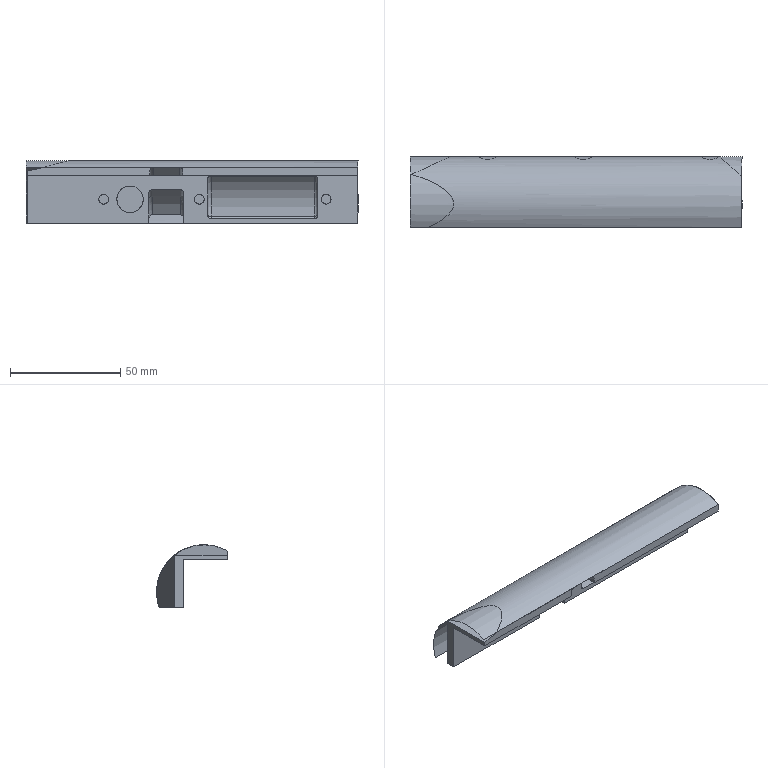NC program | Mastercam | posted with a generic post
Lines 25226 to 26102 of 52802:
(3 BM/BNOS |TOOL - 1|DIA. OFF. - 1|LEN. - 1|TOOL DIA. - 3.)
N1018 T1 M6
N1020 G0 G54 G90 X-6.118 Y-15.182 C0. B0. S6000 M3
N1022 G43 H1 Z50.
N1024 Z-20.248
N1026 G1 X-5.975 Y-15.17 Z-20.25 F2000.
N1028 X-5.578 Y-15.018 Z-20.258
N1030 X-5.28 Y-14.715 Z-20.265
N1032 X-5.135 Y-14.315 Z-20.273
N1034 X-5.126 Y-14.173 Z-20.275
N1036 X-5.128 Y-13.966
N1038 X-5.129 Y-.665
N1040 G3 X-5.128 Y-.638 I-.614 J.027
N1042 X-5.49 Y-.078 I-.615
N1044 G1 X-5.772 Y-.061
N1046 X-18.564 Y-.069
N1048 G3 X-18.907 Y-.388 I.16 J-.517
N1050 X-18.967 Y-.811 I1.449 J-.423
N1052 X-18.962 Y-.943 I1.509
N1054 G1 Y-13.966
N1056 X-18.964 Y-14.173
N1058 X-18.955 Y-14.315 Z-20.273
N1060 X-18.81 Y-14.715 Z-20.265
N1062 X-18.512 Y-15.018 Z-20.258
N1064 X-18.115 Y-15.17 Z-20.25
N1066 X-17.972 Y-15.182 Z-20.248
N1068 G0 Z50.
N1070 X-6.391 Y-15.18
N1072 Z-20.546
N1074 G1 X-6.249 Y-15.169 Z-20.548
N1076 X-5.852 Y-15.017 Z-20.556
N1078 X-5.553 Y-14.715 Z-20.563
N1080 X-5.407 Y-14.315 Z-20.571
N1082 X-5.398 Y-14.173 Z-20.573
N1084 X-5.399 Y-13.966
N1086 X-5.423 Y-.523
N1088 G3 X-5.628 Y-.332 I-.236 J-.049
N1090 G1 X-18.441
N1092 G3 X-18.667 Y-.518 I.012 J-.244
N1094 G1 X-18.689 Y-.665
N1096 X-18.692 Y-14.173
N1098 X-18.682 Y-14.315 Z-20.571
N1100 X-18.534 Y-14.714 Z-20.563
N1102 X-18.233 Y-15.014 Z-20.556
N1104 X-17.835 Y-15.163 Z-20.548
N1106 X-17.693 Y-15.173 Z-20.546
N1108 G0 Z50.
N1110 X-6.557 Y-15.179
N1112 Z-20.844
N1114 G1 X-6.415 Y-15.168 Z-20.847
N1116 X-6.017 Y-15.017 Z-20.854
N1118 X-5.719 Y-14.715 Z-20.862
N1120 X-5.573 Y-14.315 Z-20.869
N1122 X-5.563 Y-14.173 Z-20.872
N1124 X-5.564 Y-13.966
N1126 X-5.57 Y-.618
N1128 X-5.62 Y-.499
N1130 X-18.467 Y-.498
N1132 G3 X-18.524 Y-.651 I.176 J-.153
N1134 G1 Y-.665
N1136 X-18.526 Y-7.977
N1138 X-18.527 Y-14.173
N1140 X-18.517 Y-14.315 Z-20.869
N1142 X-18.369 Y-14.714 Z-20.862
N1144 X-18.068 Y-15.014 Z-20.854
N1146 X-17.67 Y-15.163 Z-20.847
N1148 X-17.527 Y-15.173 Z-20.844
N1150 G0 Z50.
N1152 X-6.65 Y-15.179
N1154 Z-21.142
N1156 G1 X-6.508 Y-15.168 Z-21.145
N1158 X-6.11 Y-15.017 Z-21.152
N1160 X-5.812 Y-14.714 Z-21.16
N1162 X-5.665 Y-14.315 Z-21.167
N1164 X-5.656 Y-14.173 Z-21.17
N1166 X-5.657 Y-13.966
N1168 X-5.662 Y-.633
N1170 X-18.428
N1172 X-18.441 Y-14.173
N1174 X-18.431 Y-14.315 Z-21.167
N1176 X-18.283 Y-14.714 Z-21.16
N1178 X-17.982 Y-15.015 Z-21.152
N1180 X-17.584 Y-15.164 Z-21.145
N1182 X-17.442 Y-15.174 Z-21.142
N1184 G0 Z50.
N1186 X-6.683 Y-15.179
N1188 Z-21.44
N1190 G1 X-6.541 Y-15.168 Z-21.443
N1192 X-6.143 Y-15.017 Z-21.45
N1194 X-5.844 Y-14.714 Z-21.458
N1196 X-5.698 Y-14.315 Z-21.465
N1198 X-5.689 Y-14.173 Z-21.468
N1200 X-5.69 Y-13.966
N1202 Y-.768
N1204 X-18.398
N1206 X-18.402 Y-14.173
N1208 X-18.392 Y-14.315 Z-21.465
N1210 X-18.243 Y-14.714 Z-21.458
N1212 X-17.943 Y-15.014 Z-21.45
N1214 X-17.544 Y-15.163 Z-21.443
N1216 X-17.402 Y-15.173 Z-21.44
N1218 G0 Z50.
N1220 X-6.688
N1222 Z-21.739
N1224 G1 X-6.546 Y-15.163 Z-21.741
N1226 X-6.148 Y-15.014 Z-21.749
N1228 X-5.847 Y-14.714 Z-21.756
N1230 X-5.699 Y-14.315 Z-21.764
N1232 X-5.688 Y-14.173 Z-21.766
N1234 X-5.69 Y-8.182
N1236 X-5.691 Y-.909
N1238 X-18.4 Y-.915
N1240 X-18.401 Y-14.173
N1242 X-18.392 Y-14.315 Z-21.764
N1244 X-18.245 Y-14.714 Z-21.756
N1246 X-17.947 Y-15.017 Z-21.749
N1248 X-17.549 Y-15.168 Z-21.741
N1250 X-17.407 Y-15.179 Z-21.739
N1252 G0 Z50.
N1254 X-6.688 Y-15.173
N1256 Z-22.037
N1258 G1 X-6.546 Y-15.163 Z-22.039
N1260 X-6.148 Y-15.014 Z-22.047
N1262 X-5.847 Y-14.714 Z-22.054
N1264 X-5.699 Y-14.315 Z-22.062
N1266 X-5.688 Y-14.173 Z-22.064
N1268 X-5.691 Y-1.059
N1270 X-18.399
N1272 X-18.402 Y-14.173
N1274 X-18.391 Y-14.315 Z-22.062
N1276 X-18.243 Y-14.714 Z-22.054
N1278 X-17.942 Y-15.014 Z-22.047
N1280 X-17.544 Y-15.163 Z-22.039
N1282 X-17.402 Y-15.173 Z-22.037
N1284 G0 Z50.
N1286 X-6.688
N1288 Z-22.335
N1290 G1 X-6.546 Y-15.163 Z-22.337
N1292 X-6.148 Y-15.014 Z-22.345
N1294 X-5.847 Y-14.714 Z-22.352
N1296 X-5.699 Y-14.315 Z-22.36
N1298 X-5.688 Y-14.173 Z-22.362
N1300 X-5.69 Y-8.332
N1302 X-5.691 Y-1.208
N1304 X-18.4 Y-1.22
N1306 X-18.401 Y-14.173
N1308 X-18.392 Y-14.315 Z-22.36
N1310 X-18.245 Y-14.714 Z-22.352
N1312 X-17.947 Y-15.017 Z-22.345
N1314 X-17.549 Y-15.168 Z-22.337
N1316 X-17.407 Y-15.179 Z-22.335
N1318 G0 Z50.
N1320 X-6.688 Y-15.173
N1322 Z-22.633
N1324 G1 X-6.546 Y-15.163 Z-22.636
N1326 X-6.148 Y-15.014 Z-22.643
N1328 X-5.847 Y-14.714 Z-22.651
N1330 X-5.699 Y-14.315 Z-22.658
N1332 X-5.688 Y-14.173 Z-22.661
N1334 X-5.69 Y-8.412
N1336 X-5.691 Y-1.368
N1338 X-18.4 Y-1.37
N1340 X-18.401 Y-14.173
N1342 X-18.392 Y-14.315 Z-22.658
N1344 X-18.245 Y-14.714 Z-22.651
N1346 X-17.947 Y-15.017 Z-22.643
N1348 X-17.549 Y-15.168 Z-22.636
N1350 X-17.407 Y-15.179 Z-22.633
N1352 G0 Z50.
N1354 X-6.688 Y-15.173
N1356 Z-22.931
N1358 G1 X-6.546 Y-15.163 Z-22.934
N1360 X-6.148 Y-15.014 Z-22.941
N1362 X-5.847 Y-14.714 Z-22.949
N1364 X-5.699 Y-14.315 Z-22.956
N1366 X-5.688 Y-14.173 Z-22.959
N1368 X-5.69 Y-1.535
N1370 X-18.4 Y-1.533
N1372 X-18.402 Y-14.173
N1374 X-18.391 Y-14.315 Z-22.956
N1376 X-18.243 Y-14.714 Z-22.949
N1378 X-17.942 Y-15.014 Z-22.941
N1380 X-17.544 Y-15.163 Z-22.934
N1382 X-17.402 Y-15.173 Z-22.931
N1384 G0 Z50.
N1386 X-6.688
N1388 Z-23.229
N1390 G1 X-6.546 Y-15.163 Z-23.232
N1392 X-6.148 Y-15.014 Z-23.239
N1394 X-5.847 Y-14.714 Z-23.247
N1396 X-5.699 Y-14.315 Z-23.254
N1398 X-5.688 Y-14.173 Z-23.257
N1400 X-5.69 Y-8.577
N1402 Y-1.7
N1404 X-18.4 Y-1.701
N1406 X-18.401 Y-14.173
N1408 X-18.392 Y-14.315 Z-23.254
N1410 X-18.245 Y-14.714 Z-23.247
N1412 X-17.947 Y-15.017 Z-23.239
N1414 X-17.549 Y-15.168 Z-23.232
N1416 X-17.407 Y-15.179 Z-23.229
N1418 G0 Z50.
N1420 X-6.688 Y-15.173
N1422 Z-23.528
N1424 G1 X-6.546 Y-15.163 Z-23.53
N1426 X-6.148 Y-15.014 Z-23.538
N1428 X-5.847 Y-14.714 Z-23.545
N1430 X-5.699 Y-14.315 Z-23.553
N1432 X-5.688 Y-14.173 Z-23.555
N1434 X-5.69 Y-8.667
N1436 Y-1.88
N1438 X-18.4
N1440 X-18.401 Y-14.173
N1442 X-18.392 Y-14.315 Z-23.553
N1444 X-18.245 Y-14.714 Z-23.545
N1446 X-17.947 Y-15.017 Z-23.538
N1448 X-17.549 Y-15.168 Z-23.53
N1450 X-17.407 Y-15.179 Z-23.528
N1452 G0 Z50.
N1454 X-6.688 Y-15.173
N1456 Z-23.826
N1458 G1 X-6.546 Y-15.163 Z-23.828
N1460 X-6.148 Y-15.014 Z-23.836
N1462 X-5.847 Y-14.714 Z-23.843
N1464 X-5.699 Y-14.315 Z-23.851
N1466 X-5.688 Y-14.173 Z-23.853
N1468 X-5.69 Y-8.758
N1470 Y-2.061
N1472 X-18.4 Y-2.064
N1474 X-18.401 Y-14.173
N1476 X-18.392 Y-14.315 Z-23.851
N1478 X-18.245 Y-14.714 Z-23.843
N1480 X-17.947 Y-15.017 Z-23.836
N1482 X-17.549 Y-15.168 Z-23.828
N1484 X-17.407 Y-15.179 Z-23.826
N1486 G0 Z50.
N1488 X-6.688 Y-15.173
N1490 Z-24.124
N1492 G1 X-6.546 Y-15.163 Z-24.126
N1494 X-6.148 Y-15.014 Z-24.134
N1496 X-5.847 Y-14.714 Z-24.141
N1498 X-5.699 Y-14.315 Z-24.149
N1500 X-5.688 Y-14.173 Z-24.151
N1502 X-5.69 Y-2.247
N1504 X-18.4
N1506 X-18.402 Y-14.173
N1508 X-18.391 Y-14.315 Z-24.149
N1510 X-18.243 Y-14.714 Z-24.141
N1512 X-17.942 Y-15.014 Z-24.134
N1514 X-17.544 Y-15.163 Z-24.126
N1516 X-17.402 Y-15.173 Z-24.124
N1518 G0 Z50.
N1520 X-6.688
N1522 Z-24.422
N1524 G1 X-6.546 Y-15.163 Z-24.425
N1526 X-6.148 Y-15.014 Z-24.432
N1528 X-5.847 Y-14.714 Z-24.44
N1530 X-5.699 Y-14.315 Z-24.447
N1532 X-5.688 Y-14.173 Z-24.45
N1534 X-5.69 Y-8.951
N1536 Y-2.449
N1538 X-18.4 Y-2.45
N1540 X-18.401 Y-14.173
N1542 X-18.392 Y-14.315 Z-24.447
N1544 X-18.245 Y-14.714 Z-24.44
N1546 X-17.947 Y-15.017 Z-24.432
N1548 X-17.549 Y-15.168 Z-24.425
N1550 X-17.407 Y-15.179 Z-24.422
N1552 G0 Z50.
N1554 X-6.688 Y-15.173
N1556 Z-24.72
N1558 G1 X-6.546 Y-15.163 Z-24.723
N1560 X-6.148 Y-15.014 Z-24.73
N1562 X-5.847 Y-14.714 Z-24.738
N1564 X-5.699 Y-14.315 Z-24.745
N1566 X-5.688 Y-14.173 Z-24.748
N1568 X-5.69 Y-9.051
N1570 Y-2.647
N1572 X-18.4 Y-2.649
N1574 X-18.401 Y-14.173
N1576 X-18.392 Y-14.315 Z-24.745
N1578 X-18.245 Y-14.714 Z-24.738
N1580 X-17.947 Y-15.017 Z-24.73
N1582 X-17.549 Y-15.168 Z-24.723
N1584 X-17.407 Y-15.179 Z-24.72
N1586 G0 Z50.
N1588 X-6.688 Y-15.173
N1590 Z-25.018
N1592 G1 X-6.546 Y-15.163 Z-25.021
N1594 X-6.148 Y-15.014 Z-25.028
N1596 X-5.847 Y-14.714 Z-25.036
N1598 X-5.699 Y-14.315 Z-25.043
N1600 X-5.688 Y-14.173 Z-25.046
N1602 X-5.691 Y-2.857
N1604 X-18.399
N1606 X-18.402 Y-14.173
N1608 X-18.391 Y-14.315 Z-25.043
N1610 X-18.243 Y-14.714 Z-25.036
N1612 X-17.942 Y-15.014 Z-25.028
N1614 X-17.544 Y-15.163 Z-25.021
N1616 X-17.402 Y-15.173 Z-25.018
N1618 G0 Z50.
N1620 X-6.688
N1622 Z-25.317
N1624 G1 X-6.546 Y-15.163 Z-25.319
N1626 X-6.148 Y-15.014 Z-25.327
N1628 X-5.847 Y-14.714 Z-25.334
N1630 X-5.699 Y-14.315 Z-25.342
N1632 X-5.688 Y-14.173 Z-25.344
N1634 X-5.691 Y-3.076
N1636 X-18.399
N1638 X-18.402 Y-14.173
N1640 X-18.391 Y-14.315 Z-25.342
N1642 X-18.243 Y-14.714 Z-25.334
N1644 X-17.942 Y-15.014 Z-25.327
N1646 X-17.544 Y-15.163 Z-25.319
N1648 X-17.402 Y-15.173 Z-25.317
N1650 G0 Z50.
N1652 X-6.688
N1654 Z-25.615
N1656 G1 X-6.546 Y-15.163 Z-25.617
N1658 X-6.148 Y-15.014 Z-25.625
N1660 X-5.847 Y-14.714 Z-25.632
N1662 X-5.699 Y-14.315 Z-25.64
N1664 X-5.688 Y-14.173 Z-25.642
N1666 X-5.69 Y-3.295
N1668 X-18.4
N1670 Y-13.966
N1672 G2 X-18.391 Y-14.136 I-1.654 J-.17
N1674 X-18.392 Y-14.173 I-1.663
N1676 G1 X-18.385 Y-14.315 Z-25.64
N1678 X-18.245 Y-14.717 Z-25.632
N1680 X-17.951 Y-15.024 Z-25.625
N1682 X-17.556 Y-15.182 Z-25.617
N1684 X-17.414 Y-15.195 Z-25.615
N1686 G0 Z50.
N1688 X-6.688 Y-15.173
N1690 Z-25.913
N1692 G1 X-6.546 Y-15.163 Z-25.915
N1694 X-6.148 Y-15.014 Z-25.923
N1696 X-5.847 Y-14.714 Z-25.93
N1698 X-5.699 Y-14.315 Z-25.938
N1700 X-5.688 Y-14.173 Z-25.94
N1702 X-5.69 Y-3.534
N1704 X-18.4 Y-3.533
N1706 Y-13.966
N1708 G2 X-18.391 Y-14.136 I-1.654 J-.17
N1710 X-18.392 Y-14.173 I-1.663
N1712 G1 X-18.385 Y-14.315 Z-25.938
N1714 X-18.245 Y-14.717 Z-25.93
N1716 X-17.951 Y-15.024 Z-25.923
N1718 X-17.556 Y-15.182 Z-25.915
N1720 X-17.414 Y-15.195 Z-25.913
N1722 G0 Z50.
N1724 X-6.688 Y-15.173
N1726 Z-26.211
N1728 G1 X-6.546 Y-15.163 Z-26.214
N1730 X-6.148 Y-15.014 Z-26.221
N1732 X-5.847 Y-14.714 Z-26.229
N1734 X-5.699 Y-14.315 Z-26.236
N1736 X-5.688 Y-14.173 Z-26.239
N1738 X-5.69 Y-3.773
N1740 X-18.4 Y-3.772
N1742 X-18.402 Y-14.173
N1744 X-18.391 Y-14.315 Z-26.236
N1746 X-18.243 Y-14.714 Z-26.229
N1748 X-17.942 Y-15.014 Z-26.221
N1750 X-17.544 Y-15.163 Z-26.214
N1752 X-17.402 Y-15.173 Z-26.211
N1754 G0 Z50.
N1756 X-6.688
N1758 Z-26.509
N1760 G1 X-6.546 Y-15.163 Z-26.512
N1762 X-6.148 Y-15.014 Z-26.519
N1764 X-5.847 Y-14.714 Z-26.527
N1766 X-5.699 Y-14.315 Z-26.534
N1768 X-5.688 Y-14.173 Z-26.537
N1770 X-5.69 Y-4.023
N1772 X-18.398 Y-4.022
N1774 X-18.4 Y-13.966
N1776 G2 X-18.391 Y-14.136 I-1.654 J-.17
N1778 X-18.392 Y-14.173 I-1.663
N1780 G1 X-18.385 Y-14.315 Z-26.534
N1782 X-18.245 Y-14.717 Z-26.527
N1784 X-17.951 Y-15.024 Z-26.519
N1786 X-17.556 Y-15.182 Z-26.512
N1788 X-17.414 Y-15.195 Z-26.509
N1790 G0 Z50.
N1792 X-6.688 Y-15.173
N1794 Z-26.807
N1796 G1 X-6.546 Y-15.163 Z-26.81
N1798 X-6.148 Y-15.014 Z-26.817
N1800 X-5.847 Y-14.714 Z-26.825
N1802 X-5.699 Y-14.315 Z-26.832
N1804 X-5.688 Y-14.173 Z-26.835
N1806 X-5.69 Y-4.284
N1808 X-18.399 Y-4.282
N1810 X-18.402 Y-14.173
N1812 X-18.391 Y-14.315 Z-26.832
N1814 X-18.243 Y-14.714 Z-26.825
N1816 X-17.942 Y-15.014 Z-26.817
N1818 X-17.544 Y-15.163 Z-26.81
N1820 X-17.402 Y-15.173 Z-26.807
N1822 G0 Z50.
N1824 X-6.688
N1826 Z-27.106
N1828 G1 X-6.546 Y-15.163 Z-27.108
N1830 X-6.148 Y-15.014 Z-27.116
N1832 X-5.847 Y-14.714 Z-27.123
N1834 X-5.699 Y-14.315 Z-27.131
N1836 X-5.688 Y-14.173 Z-27.133
N1838 X-5.69 Y-4.547
N1840 X-18.4 Y-4.545
N1842 X-18.402 Y-14.173
N1844 X-18.391 Y-14.315 Z-27.131
N1846 X-18.243 Y-14.714 Z-27.123
N1848 X-17.942 Y-15.014 Z-27.116
N1850 X-17.544 Y-15.163 Z-27.108
N1852 X-17.402 Y-15.173 Z-27.106
N1854 G0 Z50.
N1856 X-6.688
N1858 Z-27.404
N1860 G1 X-6.546 Y-15.163 Z-27.406
N1862 X-6.148 Y-15.014 Z-27.414
N1864 X-5.847 Y-14.714 Z-27.421
N1866 X-5.699 Y-14.315 Z-27.429
N1868 X-5.688 Y-14.173 Z-27.431
N1870 X-5.69 Y-4.829
N1872 X-18.398 Y-4.828
N1874 X-18.402 Y-14.173
N1876 X-18.391 Y-14.315 Z-27.429
N1878 X-18.243 Y-14.714 Z-27.421
N1880 X-17.942 Y-15.014 Z-27.414
N1882 X-17.544 Y-15.163 Z-27.406
N1884 X-17.402 Y-15.173 Z-27.404
N1886 G0 Z50.
N1888 X-6.688
N1890 Z-27.702
N1892 G1 X-6.546 Y-15.163 Z-27.704
N1894 X-6.148 Y-15.014 Z-27.712
N1896 X-5.847 Y-14.714 Z-27.719
N1898 X-5.699 Y-14.315 Z-27.727
N1900 X-5.688 Y-14.173 Z-27.729
N1902 X-5.69 Y-5.113
N1904 X-18.4 Y-5.112
N1906 X-18.402 Y-14.173
N1908 X-18.391 Y-14.315 Z-27.727
N1910 X-18.243 Y-14.714 Z-27.719
N1912 X-17.942 Y-15.014 Z-27.712
N1914 X-17.544 Y-15.163 Z-27.704
N1916 X-17.402 Y-15.173 Z-27.702
N1918 G0 Z50.
N1920 X-6.688
N1922 Z-28.
N1924 G1 X-6.546 Y-15.163 Z-28.003
N1926 X-6.148 Y-15.014 Z-28.01
N1928 X-5.847 Y-14.714 Z-28.018
N1930 X-5.699 Y-14.315 Z-28.025
N1932 X-5.688 Y-14.173 Z-28.028
N1934 X-5.69 Y-5.417
N1936 X-18.4 Y-5.416
N1938 X-18.402 Y-14.173
N1940 X-18.391 Y-14.315 Z-28.025
N1942 X-18.243 Y-14.714 Z-28.018
N1944 X-17.942 Y-15.014 Z-28.01
N1946 X-17.544 Y-15.163 Z-28.003
N1948 X-17.402 Y-15.173 Z-28.
N1950 G0 Z50.
N1952 X-6.688
N1954 Z-28.298
N1956 G1 X-6.546 Y-15.163 Z-28.301
N1958 X-6.148 Y-15.014 Z-28.308
N1960 X-5.847 Y-14.714 Z-28.316
N1962 X-5.699 Y-14.315 Z-28.323
N1964 X-5.688 Y-14.173 Z-28.326
N1966 X-5.69 Y-5.725
N1968 X-18.4
N1970 X-18.402 Y-14.173
N1972 X-18.391 Y-14.315 Z-28.323
N1974 X-18.243 Y-14.714 Z-28.316
N1976 X-17.942 Y-15.014 Z-28.308
N1978 X-17.544 Y-15.163 Z-28.301
N1980 X-17.402 Y-15.173 Z-28.298
N1982 G0 Z50.
N1984 X-6.688
N1986 Z-28.596
N1988 G1 X-6.546 Y-15.163 Z-28.599
N1990 X-6.148 Y-15.014 Z-28.606
N1992 X-5.847 Y-14.714 Z-28.614
N1994 X-5.699 Y-14.315 Z-28.621
N1996 X-5.688 Y-14.173 Z-28.624
N1998 X-5.69 Y-6.047
N2000 X-18.399
N2002 X-18.402 Y-14.173
N2004 X-18.391 Y-14.315 Z-28.621
N2006 X-18.243 Y-14.714 Z-28.614
N2008 X-17.942 Y-15.014 Z-28.606
N2010 X-17.544 Y-15.163 Z-28.599
N2012 X-17.402 Y-15.173 Z-28.596
N2014 G0 Z50.
N2016 X-6.688
N2018 Z-28.895
N2020 G1 X-6.546 Y-15.163 Z-28.897
N2022 X-6.148 Y-15.014 Z-28.905
N2024 X-5.847 Y-14.714 Z-28.912
N2026 X-5.699 Y-14.315 Z-28.92
N2028 X-5.688 Y-14.173 Z-28.922
N2030 X-5.69 Y-6.386
N2032 X-18.4 Y-6.384
N2034 X-18.402 Y-14.173
N2036 X-18.391 Y-14.315 Z-28.92
N2038 X-18.243 Y-14.714 Z-28.912
N2040 X-17.942 Y-15.014 Z-28.905
N2042 X-17.544 Y-15.163 Z-28.897
N2044 X-17.402 Y-15.173 Z-28.895
N2046 G0 Z50.
N2048 X-6.688
N2050 Z-29.193
N2052 G1 X-6.546 Y-15.163 Z-29.195
N2054 X-6.148 Y-15.014 Z-29.203
N2056 X-5.847 Y-14.714 Z-29.21
N2058 X-5.699 Y-14.315 Z-29.218
N2060 X-5.688 Y-14.173 Z-29.22
N2062 X-5.69 Y-6.736
N2064 X-18.399 Y-6.735
N2066 X-18.402 Y-14.173
N2068 X-18.391 Y-14.315 Z-29.218
N2070 X-18.243 Y-14.714 Z-29.21
N2072 X-17.942 Y-15.014 Z-29.203
N2074 X-17.544 Y-15.163 Z-29.195
N2076 X-17.402 Y-15.173 Z-29.193
N2078 G0 Z50.
N2080 X-6.688
N2082 Z-29.491
N2084 G1 X-6.546 Y-15.163 Z-29.493
N2086 X-6.148 Y-15.014 Z-29.501
N2088 X-5.847 Y-14.714 Z-29.508
N2090 X-5.699 Y-14.315 Z-29.516
N2092 X-5.688 Y-14.173 Z-29.518
N2094 X-5.69 Y-7.1
N2096 X-18.4
N2098 X-18.402 Y-14.173
N2100 X-18.391 Y-14.315 Z-29.516
N2102 X-18.243 Y-14.714 Z-29.508
N2104 X-17.942 Y-15.014 Z-29.501
N2106 X-17.544 Y-15.163 Z-29.493
N2108 X-17.402 Y-15.173 Z-29.491
N2110 G0 Z50.
N2112 X-6.688
N2114 Z-29.789
N2116 G1 X-6.546 Y-15.163 Z-29.792
N2118 X-6.148 Y-15.014 Z-29.799
N2120 X-5.847 Y-14.714 Z-29.807
N2122 X-5.699 Y-14.315 Z-29.814
N2124 X-5.688 Y-14.173 Z-29.817
N2126 X-5.69 Y-7.484
N2128 X-18.4
N2130 X-18.402 Y-14.173
N2132 X-18.391 Y-14.315 Z-29.814
N2134 X-18.243 Y-14.714 Z-29.807
N2136 X-17.942 Y-15.014 Z-29.799
N2138 X-17.544 Y-15.163 Z-29.792
N2140 X-17.402 Y-15.173 Z-29.789
N2142 G0 Z50.
N2144 X-6.688
N2146 Z-30.087
N2148 G1 X-6.546 Y-15.163 Z-30.09
N2150 X-6.148 Y-15.014 Z-30.097
N2152 X-5.847 Y-14.714 Z-30.105
N2154 X-5.699 Y-14.315 Z-30.112
N2156 X-5.688 Y-14.173 Z-30.115
N2158 X-5.69 Y-7.881
N2160 X-18.4 Y-7.883
N2162 X-18.402 Y-14.173
N2164 X-18.391 Y-14.315 Z-30.112
N2166 X-18.243 Y-14.714 Z-30.105
N2168 X-17.942 Y-15.014 Z-30.097
N2170 X-17.544 Y-15.163 Z-30.09
N2172 X-17.402 Y-15.173 Z-30.087
N2174 G0 Z50.
N2176 X-6.688
N2178 Z-30.385
N2180 G1 X-6.546 Y-15.163 Z-30.388
N2182 X-6.148 Y-15.014 Z-30.395
N2184 X-5.847 Y-14.714 Z-30.403
N2186 X-5.699 Y-14.315 Z-30.41
N2188 X-5.688 Y-14.173 Z-30.413
N2190 X-5.69 Y-8.303
N2192 X-18.4
N2194 Y-13.966
N2196 G2 X-18.391 Y-14.136 I-1.654 J-.17
N2198 X-18.392 Y-14.173 I-1.663
N2200 G1 X-18.385 Y-14.315 Z-30.41
N2202 X-18.245 Y-14.717 Z-30.403
N2204 X-17.951 Y-15.024 Z-30.395
N2206 X-17.556 Y-15.182 Z-30.388
N2208 X-17.414 Y-15.195 Z-30.385
N2210 G0 Z50.
N2212 X-6.688 Y-15.173
N2214 Z-30.684
N2216 G1 X-6.546 Y-15.163 Z-30.686
N2218 X-6.147 Y-15.014 Z-30.694
N2220 X-5.847 Y-14.714 Z-30.701
N2222 X-5.699 Y-14.315 Z-30.709
N2224 X-5.688 Y-14.173 Z-30.711
N2226 X-5.691 Y-8.738
N2228 X-18.4
N2230 X-18.402 Y-14.173
N2232 X-18.391 Y-14.315 Z-30.709
N2234 X-18.243 Y-14.714 Z-30.701
N2236 X-17.942 Y-15.014 Z-30.694
N2238 X-17.544 Y-15.163 Z-30.686
N2240 X-17.402 Y-15.173 Z-30.684
N2242 G0 Z50.
N2244 X-6.688
N2246 Z-30.982
N2248 G1 X-6.546 Y-15.163 Z-30.984
N2250 X-6.148 Y-15.014 Z-30.992
N2252 X-5.847 Y-14.714 Z-30.999
N2254 X-5.699 Y-14.315 Z-31.007
N2256 X-5.688 Y-14.173 Z-31.009
N2258 X-5.69 Y-9.209
N2260 X-18.399
N2262 X-18.402 Y-14.173
N2264 X-18.391 Y-14.315 Z-31.007
N2266 X-18.243 Y-14.714 Z-30.999
N2268 X-17.943 Y-15.014 Z-30.992
N2270 X-17.544 Y-15.163 Z-30.984
N2272 X-17.402 Y-15.173 Z-30.982
N2274 G0 Z50.
N2276 X-6.688
N2278 Z-31.28
N2280 G1 X-6.546 Y-15.163 Z-31.282
N2282 X-6.148 Y-15.014 Z-31.29
N2284 X-5.847 Y-14.714 Z-31.297
N2286 X-5.699 Y-14.315 Z-31.305
N2288 X-5.688 Y-14.173 Z-31.307
N2290 X-5.69 Y-9.696
N2292 X-18.4 Y-9.695
N2294 X-18.402 Y-14.173
N2296 X-18.391 Y-14.315 Z-31.305
N2298 X-18.243 Y-14.714 Z-31.297
N2300 X-17.942 Y-15.014 Z-31.29
N2302 X-17.544 Y-15.163 Z-31.282
N2304 X-17.402 Y-15.173 Z-31.28
N2306 G0 Z50.
N2308 X-6.688
N2310 Z-31.578
N2312 G1 X-6.546 Y-15.163 Z-31.581
N2314 X-6.148 Y-15.014 Z-31.588
N2316 X-5.847 Y-14.714 Z-31.596
N2318 X-5.699 Y-14.315 Z-31.603
N2320 X-5.688 Y-14.173 Z-31.606
N2322 X-5.69 Y-10.216
N2324 X-18.4
N2326 X-18.402 Y-14.173
N2328 X-18.391 Y-14.315 Z-31.603
N2330 X-18.243 Y-14.714 Z-31.596
N2332 X-17.942 Y-15.014 Z-31.588
N2334 X-17.544 Y-15.163 Z-31.581
N2336 X-17.402 Y-15.173 Z-31.578
N2338 G0 Z50.
N2340 X-6.688
N2342 Z-31.876
N2344 G1 X-6.546 Y-15.163 Z-31.879
N2346 X-6.147 Y-15.014 Z-31.886
N2348 X-5.847 Y-14.714 Z-31.894
N2350 X-5.699 Y-14.315 Z-31.901
N2352 X-5.688 Y-14.173 Z-31.904
N2354 X-5.69 Y-10.775
N2356 X-18.4 Y-10.774
N2358 X-18.402 Y-14.173
N2360 X-18.391 Y-14.315 Z-31.901
N2362 X-18.243 Y-14.714 Z-31.894
N2364 X-17.943 Y-15.014 Z-31.886
N2366 X-17.544 Y-15.163 Z-31.879
N2368 X-17.402 Y-15.173 Z-31.876
N2370 G0 Z50.
N2372 X-6.688
N2374 Z-32.174
N2376 G1 X-6.546 Y-15.163 Z-32.177
N2378 X-6.147 Y-15.014 Z-32.184
N2380 X-5.847 Y-14.714 Z-32.192
N2382 X-5.699 Y-14.315 Z-32.199
N2384 X-5.688 Y-14.173 Z-32.202
N2386 X-5.69 Y-11.298
N2388 X-18.398 Y-11.297
N2390 G3 X-18.424 Y-12.657 I35.921 J-1.36
N2392 X-18.392 Y-14.173 I35.947
N2394 G1 X-18.385 Y-14.315 Z-32.199
N2396 X-18.245 Y-14.717 Z-32.192
N2398 X-17.951 Y-15.024 Z-32.184
N2400 X-17.556 Y-15.182 Z-32.177
N2402 X-17.414 Y-15.195 Z-32.174
N2404 G0 Z50.
N2406 X-6.688 Y-15.174
N2408 Z-32.473
N2410 G1 X-6.545 Y-15.163 Z-32.475
N2412 X-6.147 Y-15.015 Z-32.483
N2414 X-5.847 Y-14.714 Z-32.49
N2416 X-5.699 Y-14.315 Z-32.498
N2418 X-5.688 Y-14.173 Z-32.5
N2420 X-5.69 Y-12.027
N2422 G3 X-5.685 Y-11.948 I-.63 J.079
N2424 X-5.79 Y-11.598 I-.635
N2426 G1 X-12.045
N2428 X-18.301
N2430 X-18.398 Y-11.852
N2432 X-18.401 Y-14.173
N2434 X-18.391 Y-14.315 Z-32.498
N2436 X-18.244 Y-14.714 Z-32.49
N2438 X-17.943 Y-15.015 Z-32.483
N2440 X-17.545 Y-15.164 Z-32.475
N2442 X-17.403 Y-15.175 Z-32.473
N2444 G0 Z50.
N2446 X11.999 Y4.977
N2448 Z-20.248
N2450 G1 X11.989 Y5.119 Z-20.25
N2452 X11.84 Y5.518 Z-20.258
N2454 X11.54 Y5.818 Z-20.265
N2456 X11.141 Y5.967 Z-20.273
N2458 X10.999 Y5.977 Z-20.275
N2460 X7.863
N2462 X7.883 Y-10.786
N2464 G3 X8.305 Y-11.126 I.444 J.119
N2466 G1 X31.748 Y-11.135
N2468 X55.041
N2470 G3 X55.11 Y-11.139 I.069 J.598
N2472 X55.455 Y-11.03 J.602
N2474 X55.632 Y-10.65 I-.32 J.38
N2476 G1 Y-10.641
N2478 X55.635 Y5.976
N2480 X52.486 Y5.977
N2482 X52.344 Y5.967 Z-20.273
N2484 X51.946 Y5.818 Z-20.265
N2486 X51.645 Y5.518 Z-20.258
N2488 X51.497 Y5.119 Z-20.25
N2490 X51.486 Y4.977 Z-20.248
N2492 G0 Z50.
N2494 X12.772
N2496 Z-20.546
N2498 G1 X12.762 Y5.119 Z-20.548
N2500 X12.613 Y5.518 Z-20.556
N2502 X12.313 Y5.818 Z-20.563
N2504 X11.914 Y5.967 Z-20.571
N2506 X11.772 Y5.977 Z-20.573
N2508 X8.134
N2510 X8.137 Y-10.641
N2512 X8.178 Y-10.782
N2514 X8.305 Y-10.853
N2516 X55.041 Y-10.863
N2518 X55.263 Y-10.83
N2520 G3 X55.359 Y-10.657 I-.107 J.173
N2522 G1 Y-10.641
N2524 X55.364 Y5.977
N2526 X51.726
N2528 X51.583 Y5.967 Z-20.571
N2530 X51.185 Y5.818 Z-20.563
N2532 X50.884 Y5.517 Z-20.556
N2534 X50.736 Y5.119 Z-20.548
N2536 X50.726 Y4.977 Z-20.546
N2538 G0 Z50.
N2540 X13.457
N2542 Z-20.844
N2544 G1 X13.447 Y5.119 Z-20.847
N2546 X13.298 Y5.518 Z-20.854
N2548 X12.997 Y5.818 Z-20.862
N2550 X12.599 Y5.967 Z-20.869
N2552 X12.457 Y5.977 Z-20.872
N2554 X8.305
N2556 X8.315 Y-10.687
N2558 X55.188 Y-10.679
N2560 X55.196 Y5.977
N2562 X51.044
N2564 X50.902 Y5.967 Z-20.869
N2566 X50.504 Y5.818 Z-20.862
N2568 X50.203 Y5.518 Z-20.854
N2570 X50.055 Y5.119 Z-20.847
N2572 X50.044 Y4.977 Z-20.844
N2574 X50.046 Y4.884
N2576 X50.152 Y4.244 Z-20.86
N2578 X50.393 Y3.794 Z-20.896
N2580 X50.722 Y3.533 Z-20.945
N2582 X51.091 Y3.462 Z-21.
N2584 X51.455 Y3.58 Z-21.054
N2586 X51.766 Y3.888 Z-21.101
N2588 X51.978 Y4.386 Z-21.132
N2590 X52.044 Y4.977 Z-21.142
N2592 X52.034 Y5.119 Z-21.145
N2594 X51.886 Y5.518 Z-21.152
N2596 X51.585 Y5.818 Z-21.16
N2598 X51.187 Y5.967 Z-21.167
N2600 X51.044 Y5.977 Z-21.17
N2602 X31.748
N2604 X8.393
N2606 Y-10.604
N2608 X55.102
N2610 X55.106 Y5.977
N2612 X8.405 Z-21.27
N2614 X8.415 Y-10.586 Z-21.309
N2616 X55.07 Y-10.573 Z-21.419
N2618 X55.062 Y5.977 Z-21.458
N2620 X8.426 Y5.952 Z-21.568
N2622 X8.437 Y-10.573 Z-21.607
N2624 X55.06 Z-21.718
N2626 X55.056 Y5.977 Z-21.757
N2628 X8.426 Y5.952 Z-21.867
N2630 X8.437 Y-10.573 Z-21.906
N2632 X55.06 Z-22.016
N2634 X55.056 Y5.977 Z-22.055
N2636 X8.426 Y5.952 Z-22.165
N2638 X8.437 Y-10.573 Z-22.204
N2640 X55.06 Z-22.314
N2642 X55.056 Y5.977 Z-22.353
N2644 X8.426 Y5.946 Z-22.463
N2646 X8.437 Y-10.572 Z-22.502
N2648 X55.06 Y-10.573 Z-22.612
N2650 X55.073 Y5.932 Z-22.651
N2652 X8.429 Y5.852 Z-22.761
N2654 X8.438 Y-10.572 Z-22.8
N2656 X55.062 Y-10.573 Z-22.91
N2658 X55.073 Y5.692 Z-22.949
N2660 X8.426 Y5.596 Z-23.06
N2662 X8.424 Y-10.572 Z-23.098
N2664 X55.063 Y-10.554 Z-23.209
N2666 X55.072 Y5.445 Z-23.247
N2668 X8.425 Y5.331 Z-23.358
N2670 X8.423 Y-10.558 Z-23.396
N2672 X55.063 Y-10.57 Z-23.507
N2674 X55.071 Y5.177 Z-23.545
N2676 X8.424 Y5.061 Z-23.657
N2678 X8.426 Y-10.572 Z-23.694
N2680 X55.063 Y-10.571 Z-23.806
N2682 X55.072 Y4.905 Z-23.843
N2684 X8.425 Y4.782 Z-23.956
N2686 X8.444 Y-10.572 Z-23.993
N2688 X55.061 Y-10.573 Z-24.105
N2690 X55.071 Y4.61 Z-24.141
N2692 X8.425 Y4.497 Z-24.254
N2694 X8.433 Y-10.572 Z-24.291
N2696 X55.063 Y-10.567 Z-24.403
N2698 X55.073 Y4.308 Z-24.44
N2700 X8.425 Y4.185 Z-24.553
N2702 X8.423 Y-10.572 Z-24.589
N2704 X55.063 Y-10.565 Z-24.702
N2706 X55.073 Y3.975 Z-24.737
N2708 X8.438 Y3.856 Z-24.852
N2710 X8.444 Y-10.573 Z-24.887
N2712 X55.054 Z-25.001
N2714 X55.073 Y3.638 Z-25.035
N2716 X8.435 Y3.51 Z-25.15
N2718 X8.423 Y-10.555 Z-25.185
N2720 X55.056 Y-10.573 Z-25.299
N2722 X55.07 Y3.28 Z-25.334
N2724 X8.424 Y3.14 Z-25.449
N2726 X8.429 Y-10.572 Z-25.483
N2728 X55.063 Y-10.567 Z-25.598
N2730 X55.069 Y2.898 Z-25.632
N2732 X8.428 Y2.752 Z-25.748
N2734 X8.426 Y-10.572 Z-25.781
N2736 X55.063 Y-10.573 Z-25.897
N2738 X55.073 Y2.502 Z-25.93
N2740 X8.425 Y2.334 Z-26.047
N2742 X8.424 Y-10.572 Z-26.079
N2744 X55.063 Y-10.562 Z-26.196
N2746 X55.067 Y2.066 Z-26.228
N2748 X8.442 Y1.89 Z-26.346
N2750 X8.425 Y-10.572 Z-26.377
N2752 X55.05 Y-10.573 Z-26.495
N2754 X55.072 Y1.606 Z-26.526
N2756 X8.43 Y1.416 Z-26.645
N2758 X8.428 Y-10.572 Z-26.675
N2760 X55.062 Y-10.573 Z-26.794
N2762 X55.071 Y1.117 Z-26.824
N2764 X8.443 Y.904 Z-26.944
N2766 X8.431 Y-10.572 Z-26.973
N2768 X55.048 Y-10.573 Z-27.093